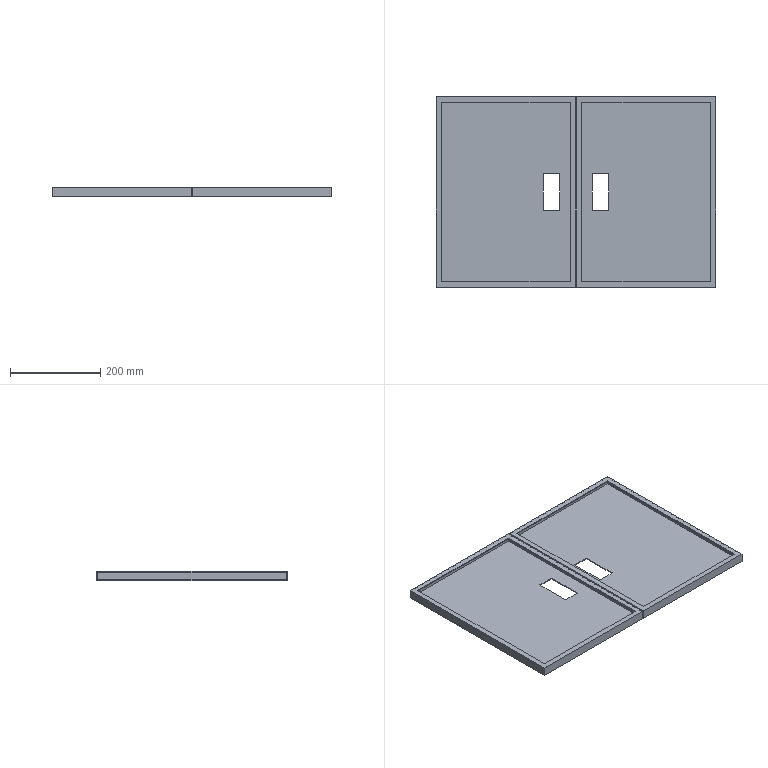Part | STEP file | Side door | 2 solids | 40 faces | box 620 x 421.75 x 20 mm | volume 670167 mm3 | plane 40